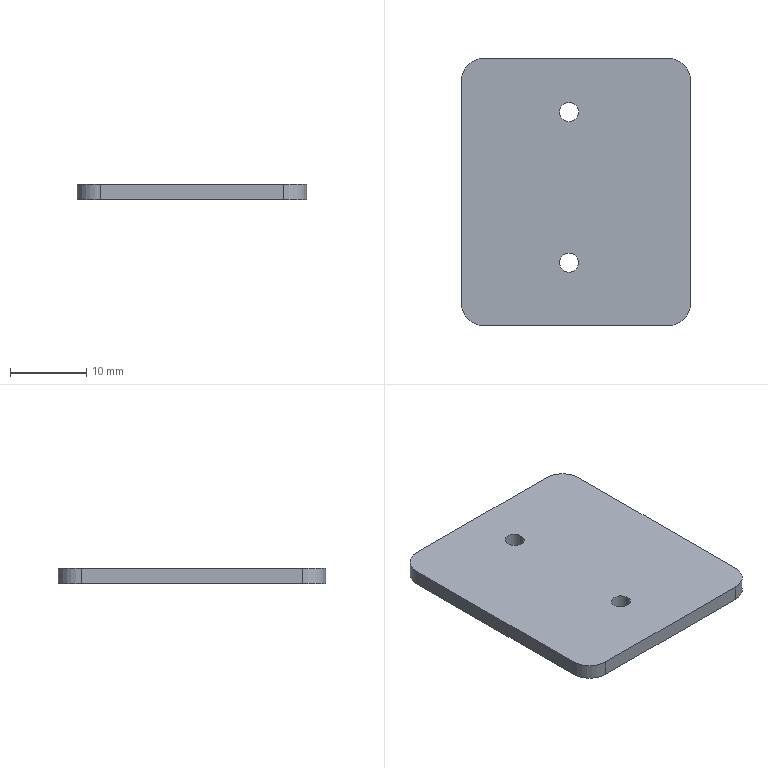Part | SolidWorks | features Extrusion 1, Fillet 1, HoleWzd 1 | 1 solid | 14 faces | box 30 x 35 x 2 mm | volume 2065 mm3 | cylinder 8 | plane 6 | commonest cylinder face diameters 2.5 x4 6 x4
STEP:
#1=CARTESIAN_POINT('',(-74.439,-40.194,0.));
#2=VERTEX_POINT('',#1);
#3=CARTESIAN_POINT('',(-71.939,-40.194,0.));
#4=VERTEX_POINT('',#3);
#5=CARTESIAN_POINT('',(-73.189,-40.194,0.));
#6=DIRECTION('',(0.,0.,1.));
#7=DIRECTION('',(1.,0.,0.));
#8=AXIS2_PLACEMENT_3D('',#5,#6,#7);
#9=CIRCLE('',#8,1.25);
#10=EDGE_CURVE('',#2,#4,#9,.T.);
#11=ORIENTED_EDGE('',*,*,#10,.F.);
#12=CARTESIAN_POINT('',(-74.439,-40.194,2.));
#13=VERTEX_POINT('',#12);
#14=CARTESIAN_POINT('',(-74.439,-40.194,2.));
#15=DIRECTION('',(0.,0.,1.));
#16=VECTOR('',#15,1000.);
#17=LINE('',#14,#16);
#18=EDGE_CURVE('',#2,#13,#17,.T.);
#19=ORIENTED_EDGE('',*,*,#18,.T.);
#20=CARTESIAN_POINT('',(-71.939,-40.194,2.));
#21=VERTEX_POINT('',#20);
#22=CARTESIAN_POINT('',(-73.189,-40.194,2.));
#23=DIRECTION('',(0.,0.,1.));
#24=DIRECTION('',(1.,0.,0.));
#25=AXIS2_PLACEMENT_3D('',#22,#23,#24);
#26=CIRCLE('',#25,1.25);
#27=EDGE_CURVE('',#13,#21,#26,.T.);
#28=ORIENTED_EDGE('',*,*,#27,.T.);
#29=CARTESIAN_POINT('',(-71.939,-40.194,2.));
#30=DIRECTION('',(0.,0.,1.));
#31=VECTOR('',#30,1000.);
#32=LINE('',#29,#31);
#33=EDGE_CURVE('',#4,#21,#32,.T.);
#34=ORIENTED_EDGE('',*,*,#33,.F.);
#35=EDGE_LOOP('',(#11,#19,#28,#34));
#36=FACE_OUTER_BOUND('',#35,.T.);
#37=CARTESIAN_POINT('',(-73.189,-40.194,2.));
#38=DIRECTION('',(0.,0.,1.));
#39=DIRECTION('',(1.,0.,0.));
#40=AXIS2_PLACEMENT_3D('',#37,#38,#39);
#41=CYLINDRICAL_SURFACE('',#40,1.25);
#42=ADVANCED_FACE('',(#36),#41,.F.);
#43=CARTESIAN_POINT('',(-74.439,-59.894,0.));
#44=VERTEX_POINT('',#43);
#45=CARTESIAN_POINT('',(-71.939,-59.894,0.));
#46=VERTEX_POINT('',#45);
#47=CARTESIAN_POINT('',(-73.189,-59.894,0.));
#48=DIRECTION('',(0.,0.,1.));
#49=DIRECTION('',(1.,0.,0.));
#50=AXIS2_PLACEMENT_3D('',#47,#48,#49);
#51=CIRCLE('',#50,1.25);
#52=EDGE_CURVE('',#44,#46,#51,.T.);
#53=ORIENTED_EDGE('',*,*,#52,.F.);
#54=CARTESIAN_POINT('',(-74.439,-59.894,2.));
#55=VERTEX_POINT('',#54);
#56=CARTESIAN_POINT('',(-74.439,-59.894,2.));
#57=DIRECTION('',(0.,0.,1.));
#58=VECTOR('',#57,1000.);
#59=LINE('',#56,#58);
#60=EDGE_CURVE('',#44,#55,#59,.T.);
#61=ORIENTED_EDGE('',*,*,#60,.T.);
#62=CARTESIAN_POINT('',(-71.939,-59.894,2.));
#63=VERTEX_POINT('',#62);
#64=CARTESIAN_POINT('',(-73.189,-59.894,2.));
#65=DIRECTION('',(0.,0.,1.));
#66=DIRECTION('',(1.,0.,0.));
#67=AXIS2_PLACEMENT_3D('',#64,#65,#66);
#68=CIRCLE('',#67,1.25);
#69=EDGE_CURVE('',#55,#63,#68,.T.);
#70=ORIENTED_EDGE('',*,*,#69,.T.);
#71=CARTESIAN_POINT('',(-71.939,-59.894,2.));
#72=DIRECTION('',(0.,0.,1.));
#73=VECTOR('',#72,1000.);
#74=LINE('',#71,#73);
#75=EDGE_CURVE('',#46,#63,#74,.T.);
#76=ORIENTED_EDGE('',*,*,#75,.F.);
#77=EDGE_LOOP('',(#53,#61,#70,#76));
#78=FACE_OUTER_BOUND('',#77,.T.);
#79=CARTESIAN_POINT('',(-73.189,-59.894,2.));
#80=DIRECTION('',(0.,0.,1.));
#81=DIRECTION('',(1.,0.,0.));
#82=AXIS2_PLACEMENT_3D('',#79,#80,#81);
#83=CYLINDRICAL_SURFACE('',#82,1.25);
#84=ADVANCED_FACE('',(#78),#83,.F.);
#85=CARTESIAN_POINT('',(-87.289,-36.155,2.));
#86=VERTEX_POINT('',#85);
#87=CARTESIAN_POINT('',(-87.289,-65.155,2.));
#88=VERTEX_POINT('',#87);
#89=CARTESIAN_POINT('',(-87.289,-33.155,2.));
#90=DIRECTION('',(0.,-1.,0.));
#91=VECTOR('',#90,1000.);
#92=LINE('',#89,#91);
#93=EDGE_CURVE('',#86,#88,#92,.T.);
#94=ORIENTED_EDGE('',*,*,#93,.F.);
#95=CARTESIAN_POINT('',(-87.289,-36.155,0.));
#96=VERTEX_POINT('',#95);
#97=CARTESIAN_POINT('',(-87.289,-36.155,2.));
#98=DIRECTION('',(0.,0.,-1.));
#99=VECTOR('',#98,1000.);
#100=LINE('',#97,#99);
#101=EDGE_CURVE('',#86,#96,#100,.T.);
#102=ORIENTED_EDGE('',*,*,#101,.T.);
#103=CARTESIAN_POINT('',(-87.289,-65.155,0.));
#104=VERTEX_POINT('',#103);
#105=CARTESIAN_POINT('',(-87.289,-33.155,0.));
#106=DIRECTION('',(0.,-1.,0.));
#107=VECTOR('',#106,1000.);
#108=LINE('',#105,#107);
#109=EDGE_CURVE('',#96,#104,#108,.T.);
#110=ORIENTED_EDGE('',*,*,#109,.T.);
#111=CARTESIAN_POINT('',(-87.289,-65.155,2.));
#112=DIRECTION('',(0.,0.,1.));
#113=VECTOR('',#112,1000.);
#114=LINE('',#111,#113);
#115=EDGE_CURVE('',#104,#88,#114,.T.);
#116=ORIENTED_EDGE('',*,*,#115,.T.);
#117=EDGE_LOOP('',(#94,#102,#110,#116));
#118=FACE_OUTER_BOUND('',#117,.T.);
#119=CARTESIAN_POINT('',(-87.289,-33.155,2.));
#120=DIRECTION('',(1.,0.,0.));
#121=DIRECTION('',(0.,1.,0.));
#122=AXIS2_PLACEMENT_3D('',#119,#120,#121);
#123=PLANE('',#122);
#124=ADVANCED_FACE('',(#118),#123,.F.);
#125=CARTESIAN_POINT('',(-84.289,-68.155,0.));
#126=VERTEX_POINT('',#125);
#127=CARTESIAN_POINT('',(-60.289,-68.155,0.));
#128=VERTEX_POINT('',#127);
#129=CARTESIAN_POINT('',(-87.289,-68.155,0.));
#130=DIRECTION('',(1.,0.,0.));
#131=VECTOR('',#130,1000.);
#132=LINE('',#129,#131);
#133=EDGE_CURVE('',#126,#128,#132,.T.);
#134=ORIENTED_EDGE('',*,*,#133,.T.);
#135=CARTESIAN_POINT('',(-60.289,-68.155,2.));
#136=VERTEX_POINT('',#135);
#137=CARTESIAN_POINT('',(-60.289,-68.155,2.));
#138=DIRECTION('',(0.,0.,1.));
#139=VECTOR('',#138,1000.);
#140=LINE('',#137,#139);
#141=EDGE_CURVE('',#128,#136,#140,.T.);
#142=ORIENTED_EDGE('',*,*,#141,.T.);
#143=CARTESIAN_POINT('',(-84.289,-68.155,2.));
#144=VERTEX_POINT('',#143);
#145=CARTESIAN_POINT('',(-87.289,-68.155,2.));
#146=DIRECTION('',(1.,0.,0.));
#147=VECTOR('',#146,1000.);
#148=LINE('',#145,#147);
#149=EDGE_CURVE('',#144,#136,#148,.T.);
#150=ORIENTED_EDGE('',*,*,#149,.F.);
#151=CARTESIAN_POINT('',(-84.289,-68.155,2.));
#152=DIRECTION('',(0.,0.,-1.));
#153=VECTOR('',#152,1000.);
#154=LINE('',#151,#153);
#155=EDGE_CURVE('',#144,#126,#154,.T.);
#156=ORIENTED_EDGE('',*,*,#155,.T.);
#157=EDGE_LOOP('',(#134,#142,#150,#156));
#158=FACE_OUTER_BOUND('',#157,.T.);
#159=CARTESIAN_POINT('',(-87.289,-68.155,2.));
#160=DIRECTION('',(0.,1.,0.));
#161=DIRECTION('',(-1.,0.,0.));
#162=AXIS2_PLACEMENT_3D('',#159,#160,#161);
#163=PLANE('',#162);
#164=ADVANCED_FACE('',(#158),#163,.F.);
#165=CARTESIAN_POINT('',(-57.289,-65.155,2.));
#166=VERTEX_POINT('',#165);
#167=CARTESIAN_POINT('',(-57.289,-36.155,2.));
#168=VERTEX_POINT('',#167);
#169=CARTESIAN_POINT('',(-57.289,-33.155,2.));
#170=DIRECTION('',(0.,1.,0.));
#171=VECTOR('',#170,1000.);
#172=LINE('',#169,#171);
#173=EDGE_CURVE('',#166,#168,#172,.T.);
#174=ORIENTED_EDGE('',*,*,#173,.F.);
#175=CARTESIAN_POINT('',(-57.289,-65.155,0.));
#176=VERTEX_POINT('',#175);
#177=CARTESIAN_POINT('',(-57.289,-65.155,2.));
#178=DIRECTION('',(0.,0.,-1.));
#179=VECTOR('',#178,1000.);
#180=LINE('',#177,#179);
#181=EDGE_CURVE('',#166,#176,#180,.T.);
#182=ORIENTED_EDGE('',*,*,#181,.T.);
#183=CARTESIAN_POINT('',(-57.289,-36.155,0.));
#184=VERTEX_POINT('',#183);
#185=CARTESIAN_POINT('',(-57.289,-33.155,0.));
#186=DIRECTION('',(0.,1.,0.));
#187=VECTOR('',#186,1000.);
#188=LINE('',#185,#187);
#189=EDGE_CURVE('',#176,#184,#188,.T.);
#190=ORIENTED_EDGE('',*,*,#189,.T.);
#191=CARTESIAN_POINT('',(-57.289,-36.155,2.));
#192=DIRECTION('',(0.,0.,1.));
#193=VECTOR('',#192,1000.);
#194=LINE('',#191,#193);
#195=EDGE_CURVE('',#184,#168,#194,.T.);
#196=ORIENTED_EDGE('',*,*,#195,.T.);
#197=EDGE_LOOP('',(#174,#182,#190,#196));
#198=FACE_OUTER_BOUND('',#197,.T.);
#199=CARTESIAN_POINT('',(-57.289,-33.155,2.));
#200=DIRECTION('',(-1.,0.,0.));
#201=DIRECTION('',(0.,-1.,0.));
#202=AXIS2_PLACEMENT_3D('',#199,#200,#201);
#203=PLANE('',#202);
#204=ADVANCED_FACE('',(#198),#203,.F.);
#205=CARTESIAN_POINT('',(-60.289,-33.155,2.));
#206=VERTEX_POINT('',#205);
#207=CARTESIAN_POINT('',(-84.289,-33.155,2.));
#208=VERTEX_POINT('',#207);
#209=CARTESIAN_POINT('',(-87.289,-33.155,2.));
#210=DIRECTION('',(-1.,0.,0.));
#211=VECTOR('',#210,1000.);
#212=LINE('',#209,#211);
#213=EDGE_CURVE('',#206,#208,#212,.T.);
#214=ORIENTED_EDGE('',*,*,#213,.F.);
#215=CARTESIAN_POINT('',(-60.289,-33.155,0.));
#216=VERTEX_POINT('',#215);
#217=CARTESIAN_POINT('',(-60.289,-33.155,2.));
#218=DIRECTION('',(0.,0.,-1.));
#219=VECTOR('',#218,1000.);
#220=LINE('',#217,#219);
#221=EDGE_CURVE('',#206,#216,#220,.T.);
#222=ORIENTED_EDGE('',*,*,#221,.T.);
#223=CARTESIAN_POINT('',(-84.289,-33.155,0.));
#224=VERTEX_POINT('',#223);
#225=CARTESIAN_POINT('',(-87.289,-33.155,0.));
#226=DIRECTION('',(-1.,0.,0.));
#227=VECTOR('',#226,1000.);
#228=LINE('',#225,#227);
#229=EDGE_CURVE('',#216,#224,#228,.T.);
#230=ORIENTED_EDGE('',*,*,#229,.T.);
#231=CARTESIAN_POINT('',(-84.289,-33.155,2.));
#232=DIRECTION('',(0.,0.,1.));
#233=VECTOR('',#232,1000.);
#234=LINE('',#231,#233);
#235=EDGE_CURVE('',#224,#208,#234,.T.);
#236=ORIENTED_EDGE('',*,*,#235,.T.);
#237=EDGE_LOOP('',(#214,#222,#230,#236));
#238=FACE_OUTER_BOUND('',#237,.T.);
#239=CARTESIAN_POINT('',(-87.289,-33.155,2.));
#240=DIRECTION('',(0.,-1.,0.));
#241=DIRECTION('',(0.,0.,-1.));
#242=AXIS2_PLACEMENT_3D('',#239,#240,#241);
#243=PLANE('',#242);
#244=ADVANCED_FACE('',(#238),#243,.F.);
#245=CARTESIAN_POINT('',(-73.189,-40.194,2.));
#246=DIRECTION('',(0.,0.,1.));
#247=DIRECTION('',(1.,0.,0.));
#248=AXIS2_PLACEMENT_3D('',#245,#246,#247);
#249=CIRCLE('',#248,1.25);
#250=EDGE_CURVE('',#21,#13,#249,.T.);
#251=ORIENTED_EDGE('',*,*,#250,.F.);
#252=ORIENTED_EDGE('',*,*,#27,.F.);
#253=EDGE_LOOP('',(#251,#252));
#254=FACE_BOUND('',#253,.T.);
#255=CARTESIAN_POINT('',(-73.189,-59.894,2.));
#256=DIRECTION('',(0.,0.,1.));
#257=DIRECTION('',(1.,0.,0.));
#258=AXIS2_PLACEMENT_3D('',#255,#256,#257);
#259=CIRCLE('',#258,1.25);
#260=EDGE_CURVE('',#63,#55,#259,.T.);
#261=ORIENTED_EDGE('',*,*,#260,.F.);
#262=ORIENTED_EDGE('',*,*,#69,.F.);
#263=EDGE_LOOP('',(#261,#262));
#264=FACE_BOUND('',#263,.T.);
#265=ORIENTED_EDGE('',*,*,#149,.T.);
#266=CARTESIAN_POINT('',(-60.289,-65.155,2.));
#267=DIRECTION('',(0.,0.,1.));
#268=DIRECTION('',(1.,0.,0.));
#269=AXIS2_PLACEMENT_3D('',#266,#267,#268);
#270=CIRCLE('',#269,3.);
#271=EDGE_CURVE('',#136,#166,#270,.T.);
#272=ORIENTED_EDGE('',*,*,#271,.T.);
#273=ORIENTED_EDGE('',*,*,#173,.T.);
#274=CARTESIAN_POINT('',(-60.289,-36.155,2.));
#275=DIRECTION('',(0.,0.,1.));
#276=DIRECTION('',(1.,0.,0.));
#277=AXIS2_PLACEMENT_3D('',#274,#275,#276);
#278=CIRCLE('',#277,3.);
#279=EDGE_CURVE('',#168,#206,#278,.T.);
#280=ORIENTED_EDGE('',*,*,#279,.T.);
#281=ORIENTED_EDGE('',*,*,#213,.T.);
#282=CARTESIAN_POINT('',(-84.289,-36.155,2.));
#283=DIRECTION('',(0.,0.,1.));
#284=DIRECTION('',(1.,0.,0.));
#285=AXIS2_PLACEMENT_3D('',#282,#283,#284);
#286=CIRCLE('',#285,3.);
#287=EDGE_CURVE('',#208,#86,#286,.T.);
#288=ORIENTED_EDGE('',*,*,#287,.T.);
#289=ORIENTED_EDGE('',*,*,#93,.T.);
#290=CARTESIAN_POINT('',(-84.289,-65.155,2.));
#291=DIRECTION('',(0.,0.,1.));
#292=DIRECTION('',(1.,0.,0.));
#293=AXIS2_PLACEMENT_3D('',#290,#291,#292);
#294=CIRCLE('',#293,3.);
#295=EDGE_CURVE('',#88,#144,#294,.T.);
#296=ORIENTED_EDGE('',*,*,#295,.T.);
#297=EDGE_LOOP('',(#265,#272,#273,#280,#281,#288,#289,#296));
#298=FACE_OUTER_BOUND('',#297,.T.);
#299=CARTESIAN_POINT('',(0.,0.,2.));
#300=DIRECTION('',(0.,0.,1.));
#301=DIRECTION('',(1.,0.,0.));
#302=AXIS2_PLACEMENT_3D('',#299,#300,#301);
#303=PLANE('',#302);
#304=ADVANCED_FACE('',(#254,#264,#298),#303,.T.);
#305=CARTESIAN_POINT('',(-73.189,-40.194,0.));
#306=DIRECTION('',(0.,0.,1.));
#307=DIRECTION('',(1.,0.,0.));
#308=AXIS2_PLACEMENT_3D('',#305,#306,#307);
#309=CIRCLE('',#308,1.25);
#310=EDGE_CURVE('',#4,#2,#309,.T.);
#311=ORIENTED_EDGE('',*,*,#310,.T.);
#312=ORIENTED_EDGE('',*,*,#10,.T.);
#313=EDGE_LOOP('',(#311,#312));
#314=FACE_BOUND('',#313,.T.);
#315=CARTESIAN_POINT('',(-73.189,-59.894,0.));
#316=DIRECTION('',(0.,0.,1.));
#317=DIRECTION('',(1.,0.,0.));
#318=AXIS2_PLACEMENT_3D('',#315,#316,#317);
#319=CIRCLE('',#318,1.25);
#320=EDGE_CURVE('',#46,#44,#319,.T.);
#321=ORIENTED_EDGE('',*,*,#320,.T.);
#322=ORIENTED_EDGE('',*,*,#52,.T.);
#323=EDGE_LOOP('',(#321,#322));
#324=FACE_BOUND('',#323,.T.);
#325=ORIENTED_EDGE('',*,*,#189,.F.);
#326=CARTESIAN_POINT('',(-60.289,-65.155,0.));
#327=DIRECTION('',(0.,0.,-1.));
#328=DIRECTION('',(1.,0.,0.));
#329=AXIS2_PLACEMENT_3D('',#326,#327,#328);
#330=CIRCLE('',#329,3.);
#331=EDGE_CURVE('',#176,#128,#330,.T.);
#332=ORIENTED_EDGE('',*,*,#331,.T.);
#333=ORIENTED_EDGE('',*,*,#133,.F.);
#334=CARTESIAN_POINT('',(-84.289,-65.155,0.));
#335=DIRECTION('',(0.,0.,-1.));
#336=DIRECTION('',(1.,0.,0.));
#337=AXIS2_PLACEMENT_3D('',#334,#335,#336);
#338=CIRCLE('',#337,3.);
#339=EDGE_CURVE('',#126,#104,#338,.T.);
#340=ORIENTED_EDGE('',*,*,#339,.T.);
#341=ORIENTED_EDGE('',*,*,#109,.F.);
#342=CARTESIAN_POINT('',(-84.289,-36.155,0.));
#343=DIRECTION('',(0.,0.,-1.));
#344=DIRECTION('',(1.,0.,0.));
#345=AXIS2_PLACEMENT_3D('',#342,#343,#344);
#346=CIRCLE('',#345,3.);
#347=EDGE_CURVE('',#96,#224,#346,.T.);
#348=ORIENTED_EDGE('',*,*,#347,.T.);
#349=ORIENTED_EDGE('',*,*,#229,.F.);
#350=CARTESIAN_POINT('',(-60.289,-36.155,0.));
#351=DIRECTION('',(0.,0.,-1.));
#352=DIRECTION('',(1.,0.,0.));
#353=AXIS2_PLACEMENT_3D('',#350,#351,#352);
#354=CIRCLE('',#353,3.);
#355=EDGE_CURVE('',#216,#184,#354,.T.);
#356=ORIENTED_EDGE('',*,*,#355,.T.);
#357=EDGE_LOOP('',(#325,#332,#333,#340,#341,#348,#349,#356));
#358=FACE_OUTER_BOUND('',#357,.T.);
#359=CARTESIAN_POINT('',(0.,0.,0.));
#360=DIRECTION('',(0.,0.,1.));
#361=DIRECTION('',(1.,0.,0.));
#362=AXIS2_PLACEMENT_3D('',#359,#360,#361);
#363=PLANE('',#362);
#364=ADVANCED_FACE('',(#314,#324,#358),#363,.F.);
#365=ORIENTED_EDGE('',*,*,#271,.F.);
#366=ORIENTED_EDGE('',*,*,#141,.F.);
#367=ORIENTED_EDGE('',*,*,#331,.F.);
#368=ORIENTED_EDGE('',*,*,#181,.F.);
#369=EDGE_LOOP('',(#365,#366,#367,#368));
#370=FACE_OUTER_BOUND('',#369,.T.);
#371=CARTESIAN_POINT('',(-60.289,-65.155,2.));
#372=DIRECTION('',(0.,0.,-1.));
#373=DIRECTION('',(-1.,0.,0.));
#374=AXIS2_PLACEMENT_3D('',#371,#372,#373);
#375=CYLINDRICAL_SURFACE('',#374,3.);
#376=ADVANCED_FACE('',(#370),#375,.T.);
#377=ORIENTED_EDGE('',*,*,#279,.F.);
#378=ORIENTED_EDGE('',*,*,#195,.F.);
#379=ORIENTED_EDGE('',*,*,#355,.F.);
#380=ORIENTED_EDGE('',*,*,#221,.F.);
#381=EDGE_LOOP('',(#377,#378,#379,#380));
#382=FACE_OUTER_BOUND('',#381,.T.);
#383=CARTESIAN_POINT('',(-60.289,-36.155,2.));
#384=DIRECTION('',(0.,0.,-1.));
#385=DIRECTION('',(-1.,0.,0.));
#386=AXIS2_PLACEMENT_3D('',#383,#384,#385);
#387=CYLINDRICAL_SURFACE('',#386,3.);
#388=ADVANCED_FACE('',(#382),#387,.T.);
#389=ORIENTED_EDGE('',*,*,#287,.F.);
#390=ORIENTED_EDGE('',*,*,#235,.F.);
#391=ORIENTED_EDGE('',*,*,#347,.F.);
#392=ORIENTED_EDGE('',*,*,#101,.F.);
#393=EDGE_LOOP('',(#389,#390,#391,#392));
#394=FACE_OUTER_BOUND('',#393,.T.);
#395=CARTESIAN_POINT('',(-84.289,-36.155,2.));
#396=DIRECTION('',(0.,0.,-1.));
#397=DIRECTION('',(-1.,0.,0.));
#398=AXIS2_PLACEMENT_3D('',#395,#396,#397);
#399=CYLINDRICAL_SURFACE('',#398,3.);
#400=ADVANCED_FACE('',(#394),#399,.T.);
#401=ORIENTED_EDGE('',*,*,#295,.F.);
#402=ORIENTED_EDGE('',*,*,#115,.F.);
#403=ORIENTED_EDGE('',*,*,#339,.F.);
#404=ORIENTED_EDGE('',*,*,#155,.F.);
#405=EDGE_LOOP('',(#401,#402,#403,#404));
#406=FACE_OUTER_BOUND('',#405,.T.);
#407=CARTESIAN_POINT('',(-84.289,-65.155,2.));
#408=DIRECTION('',(0.,0.,-1.));
#409=DIRECTION('',(-1.,0.,0.));
#410=AXIS2_PLACEMENT_3D('',#407,#408,#409);
#411=CYLINDRICAL_SURFACE('',#410,3.);
#412=ADVANCED_FACE('',(#406),#411,.T.);
#413=ORIENTED_EDGE('',*,*,#60,.F.);
#414=ORIENTED_EDGE('',*,*,#320,.F.);
#415=ORIENTED_EDGE('',*,*,#75,.T.);
#416=ORIENTED_EDGE('',*,*,#260,.T.);
#417=EDGE_LOOP('',(#413,#414,#415,#416));
#418=FACE_OUTER_BOUND('',#417,.T.);
#419=CARTESIAN_POINT('',(-73.189,-59.894,2.));
#420=DIRECTION('',(0.,0.,1.));
#421=DIRECTION('',(1.,0.,0.));
#422=AXIS2_PLACEMENT_3D('',#419,#420,#421);
#423=CYLINDRICAL_SURFACE('',#422,1.25);
#424=ADVANCED_FACE('',(#418),#423,.F.);
#425=ORIENTED_EDGE('',*,*,#18,.F.);
#426=ORIENTED_EDGE('',*,*,#310,.F.);
#427=ORIENTED_EDGE('',*,*,#33,.T.);
#428=ORIENTED_EDGE('',*,*,#250,.T.);
#429=EDGE_LOOP('',(#425,#426,#427,#428));
#430=FACE_OUTER_BOUND('',#429,.T.);
#431=CARTESIAN_POINT('',(-73.189,-40.194,2.));
#432=DIRECTION('',(0.,0.,1.));
#433=DIRECTION('',(1.,0.,0.));
#434=AXIS2_PLACEMENT_3D('',#431,#432,#433);
#435=CYLINDRICAL_SURFACE('',#434,1.25);
#436=ADVANCED_FACE('',(#430),#435,.F.);
#437=CLOSED_SHELL('',(#42,#84,#124,#164,#204,#244,#304,#364,#376,#388,#400,#412,#424,#436));
#438=MANIFOLD_SOLID_BREP('',#437);
#439=CARTESIAN_POINT('',(0.,0.,0.));
#440=DIRECTION('',(0.,0.,1.));
#441=DIRECTION('',(1.,0.,0.));
#442=AXIS2_PLACEMENT_3D('',#439,#440,#441);
#443=(LENGTH_UNIT()NAMED_UNIT(*)SI_UNIT(.MILLI.,.METRE.));
#444=UNCERTAINTY_MEASURE_WITH_UNIT(LENGTH_MEASURE(0.00001),#443,'','');
#445=(NAMED_UNIT(*)PLANE_ANGLE_UNIT()SI_UNIT($,.RADIAN.));
#446=(NAMED_UNIT(*)SI_UNIT($,.STERADIAN.)SOLID_ANGLE_UNIT());
#447=(GEOMETRIC_REPRESENTATION_CONTEXT(3)GLOBAL_UNCERTAINTY_ASSIGNED_CONTEXT((#444))GLOBAL_UNIT_ASSIGNED_CONTEXT((#443,#445,#446))REPRESENTATION_CONTEXT('',''));
#448=ADVANCED_BREP_SHAPE_REPRESENTATION('',(#438,#442),#447);